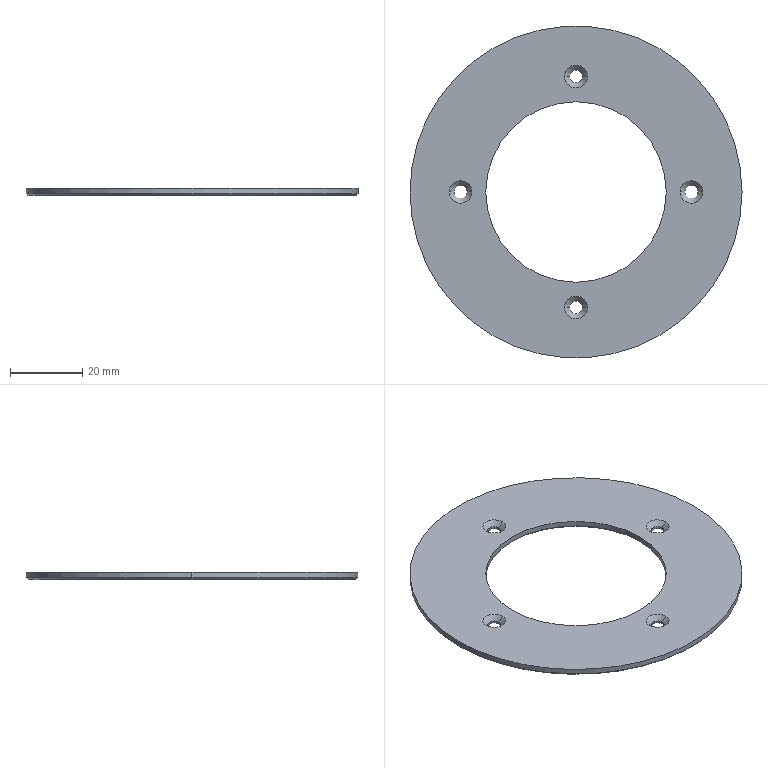Part | NX | features BREP 1 | 1 solid | 26 faces | box 92 x 92 x 2 mm | volume 9180 mm3 | cone 12 | cylinder 12 | plane 2 | commonest cylinder face diameters 3.6 x8 50 x2 92 x2
STEP:
#1=CARTESIAN_POINT('',(-45.5,0.,0.));
#2=VERTEX_POINT('',#1);
#3=CARTESIAN_POINT('',(45.5,0.,0.));
#4=VERTEX_POINT('',#3);
#5=CARTESIAN_POINT('',(0.,0.,0.));
#6=DIRECTION('',(0.,0.,-1.));
#7=DIRECTION('',(1.,0.,0.));
#8=AXIS2_PLACEMENT_3D('',#5,#6,#7);
#9=CIRCLE('',#8,45.5);
#10=EDGE_CURVE('',#2,#4,#9,.T.);
#11=ORIENTED_EDGE('',*,*,#10,.F.);
#12=CARTESIAN_POINT('',(-46.,0.,0.5));
#13=VERTEX_POINT('',#12);
#14=CARTESIAN_POINT('',(-46.,0.,0.5));
#15=DIRECTION('',(-0.7071,0.,0.7071));
#16=VECTOR('',#15,1000.);
#17=LINE('',#14,#16);
#18=EDGE_CURVE('',#13,#2,#17,.F.);
#19=ORIENTED_EDGE('',*,*,#18,.F.);
#20=CARTESIAN_POINT('',(46.,0.,0.5));
#21=VERTEX_POINT('',#20);
#22=CARTESIAN_POINT('',(0.,0.,0.5));
#23=DIRECTION('',(0.,0.,1.));
#24=DIRECTION('',(1.,0.,0.));
#25=AXIS2_PLACEMENT_3D('',#22,#23,#24);
#26=CIRCLE('',#25,46.);
#27=EDGE_CURVE('',#21,#13,#26,.T.);
#28=ORIENTED_EDGE('',*,*,#27,.F.);
#29=CARTESIAN_POINT('',(46.,0.,0.5));
#30=DIRECTION('',(0.7071,0.,0.7071));
#31=VECTOR('',#30,1000.);
#32=LINE('',#29,#31);
#33=EDGE_CURVE('',#21,#4,#32,.F.);
#34=ORIENTED_EDGE('',*,*,#33,.T.);
#35=EDGE_LOOP('',(#11,#19,#28,#34));
#36=FACE_BOUND('',#35,.T.);
#37=CARTESIAN_POINT('',(0.,0.,0.5));
#38=DIRECTION('',(0.,0.,1.));
#39=DIRECTION('',(1.,0.,0.));
#40=AXIS2_PLACEMENT_3D('',#37,#38,#39);
#41=CONICAL_SURFACE('',#40,46.,0.7854);
#42=ADVANCED_FACE('',(#36),#41,.T.);
#43=CARTESIAN_POINT('',(25.,0.,0.5));
#44=VERTEX_POINT('',#43);
#45=CARTESIAN_POINT('',(-25.,0.,0.5));
#46=VERTEX_POINT('',#45);
#47=CARTESIAN_POINT('',(0.,0.,0.5));
#48=DIRECTION('',(0.,0.,-1.));
#49=DIRECTION('',(1.,0.,0.));
#50=AXIS2_PLACEMENT_3D('',#47,#48,#49);
#51=CIRCLE('',#50,25.);
#52=EDGE_CURVE('',#44,#46,#51,.T.);
#53=ORIENTED_EDGE('',*,*,#52,.F.);
#54=CARTESIAN_POINT('',(25.5,0.,0.));
#55=VERTEX_POINT('',#54);
#56=CARTESIAN_POINT('',(25.5,0.,0.));
#57=DIRECTION('',(0.7071,0.,-0.7071));
#58=VECTOR('',#57,1000.);
#59=LINE('',#56,#58);
#60=EDGE_CURVE('',#44,#55,#59,.T.);
#61=ORIENTED_EDGE('',*,*,#60,.T.);
#62=CARTESIAN_POINT('',(-25.5,0.,0.));
#63=VERTEX_POINT('',#62);
#64=CARTESIAN_POINT('',(0.,0.,0.));
#65=DIRECTION('',(0.,0.,1.));
#66=DIRECTION('',(1.,0.,0.));
#67=AXIS2_PLACEMENT_3D('',#64,#65,#66);
#68=CIRCLE('',#67,25.5);
#69=EDGE_CURVE('',#63,#55,#68,.T.);
#70=ORIENTED_EDGE('',*,*,#69,.F.);
#71=CARTESIAN_POINT('',(-25.5,0.,0.));
#72=DIRECTION('',(-0.7071,0.,-0.7071));
#73=VECTOR('',#72,1000.);
#74=LINE('',#71,#73);
#75=EDGE_CURVE('',#46,#63,#74,.T.);
#76=ORIENTED_EDGE('',*,*,#75,.F.);
#77=EDGE_LOOP('',(#53,#61,#70,#76));
#78=FACE_BOUND('',#77,.T.);
#79=CARTESIAN_POINT('',(0.,0.,0.));
#80=DIRECTION('',(0.,0.,-1.));
#81=DIRECTION('',(-1.,0.,0.));
#82=AXIS2_PLACEMENT_3D('',#79,#80,#81);
#83=CONICAL_SURFACE('',#82,25.5,0.7854);
#84=ADVANCED_FACE('',(#78),#83,.F.);
#85=CARTESIAN_POINT('',(-33.8,0.,0.65));
#86=VERTEX_POINT('',#85);
#87=CARTESIAN_POINT('',(-30.2,0.,0.65));
#88=VERTEX_POINT('',#87);
#89=CARTESIAN_POINT('',(-32.,0.,0.65));
#90=DIRECTION('',(0.,0.,1.));
#91=DIRECTION('',(1.,0.,0.));
#92=AXIS2_PLACEMENT_3D('',#89,#90,#91);
#93=CIRCLE('',#92,1.8);
#94=EDGE_CURVE('',#86,#88,#93,.T.);
#95=ORIENTED_EDGE('',*,*,#94,.F.);
#96=CARTESIAN_POINT('',(-35.15,0.,2.));
#97=VERTEX_POINT('',#96);
#98=CARTESIAN_POINT('',(-35.15,0.,2.));
#99=DIRECTION('',(-0.7071,0.,0.7071));
#100=VECTOR('',#99,1000.);
#101=LINE('',#98,#100);
#102=EDGE_CURVE('',#97,#86,#101,.F.);
#103=ORIENTED_EDGE('',*,*,#102,.F.);
#104=CARTESIAN_POINT('',(-28.85,0.,2.));
#105=VERTEX_POINT('',#104);
#106=CARTESIAN_POINT('',(-32.,0.,2.));
#107=DIRECTION('',(0.,0.,1.));
#108=DIRECTION('',(1.,0.,0.));
#109=AXIS2_PLACEMENT_3D('',#106,#107,#108);
#110=CIRCLE('',#109,3.15);
#111=EDGE_CURVE('',#97,#105,#110,.T.);
#112=ORIENTED_EDGE('',*,*,#111,.T.);
#113=CARTESIAN_POINT('',(-28.85,0.,2.));
#114=DIRECTION('',(0.7071,0.,0.7071));
#115=VECTOR('',#114,1000.);
#116=LINE('',#113,#115);
#117=EDGE_CURVE('',#105,#88,#116,.F.);
#118=ORIENTED_EDGE('',*,*,#117,.T.);
#119=EDGE_LOOP('',(#95,#103,#112,#118));
#120=FACE_BOUND('',#119,.T.);
#121=CARTESIAN_POINT('',(-32.,0.,2.));
#122=DIRECTION('',(0.,0.,1.));
#123=DIRECTION('',(1.,0.,0.));
#124=AXIS2_PLACEMENT_3D('',#121,#122,#123);
#125=CONICAL_SURFACE('',#124,3.15,0.7854);
#126=ADVANCED_FACE('',(#120),#125,.F.);
#127=CARTESIAN_POINT('',(-33.8,0.,0.));
#128=VERTEX_POINT('',#127);
#129=CARTESIAN_POINT('',(-30.2,0.,0.));
#130=VERTEX_POINT('',#129);
#131=CARTESIAN_POINT('',(-32.,0.,0.));
#132=DIRECTION('',(0.,0.,1.));
#133=DIRECTION('',(1.,0.,0.));
#134=AXIS2_PLACEMENT_3D('',#131,#132,#133);
#135=CIRCLE('',#134,1.8);
#136=EDGE_CURVE('',#128,#130,#135,.T.);
#137=ORIENTED_EDGE('',*,*,#136,.F.);
#138=CARTESIAN_POINT('',(-33.8,0.,2.));
#139=DIRECTION('',(0.,0.,1.));
#140=VECTOR('',#139,1000.);
#141=LINE('',#138,#140);
#142=EDGE_CURVE('',#86,#128,#141,.F.);
#143=ORIENTED_EDGE('',*,*,#142,.F.);
#144=ORIENTED_EDGE('',*,*,#94,.T.);
#145=CARTESIAN_POINT('',(-30.2,0.,2.));
#146=DIRECTION('',(0.,0.,1.));
#147=VECTOR('',#146,1000.);
#148=LINE('',#145,#147);
#149=EDGE_CURVE('',#88,#130,#148,.F.);
#150=ORIENTED_EDGE('',*,*,#149,.T.);
#151=EDGE_LOOP('',(#137,#143,#144,#150));
#152=FACE_BOUND('',#151,.T.);
#153=CARTESIAN_POINT('',(-32.,0.,2.));
#154=DIRECTION('',(0.,0.,1.));
#155=DIRECTION('',(1.,0.,0.));
#156=AXIS2_PLACEMENT_3D('',#153,#154,#155);
#157=CYLINDRICAL_SURFACE('',#156,1.8);
#158=ADVANCED_FACE('',(#152),#157,.F.);
#159=CARTESIAN_POINT('',(-1.8,-32.,0.65));
#160=VERTEX_POINT('',#159);
#161=CARTESIAN_POINT('',(1.8,-32.,0.65));
#162=VERTEX_POINT('',#161);
#163=CARTESIAN_POINT('',(0.,-32.,0.65));
#164=DIRECTION('',(0.,0.,1.));
#165=DIRECTION('',(1.,0.,0.));
#166=AXIS2_PLACEMENT_3D('',#163,#164,#165);
#167=CIRCLE('',#166,1.8);
#168=EDGE_CURVE('',#160,#162,#167,.T.);
#169=ORIENTED_EDGE('',*,*,#168,.F.);
#170=CARTESIAN_POINT('',(-3.15,-32.,2.));
#171=VERTEX_POINT('',#170);
#172=CARTESIAN_POINT('',(-3.15,-32.,2.));
#173=DIRECTION('',(-0.7071,0.,0.7071));
#174=VECTOR('',#173,1000.);
#175=LINE('',#172,#174);
#176=EDGE_CURVE('',#171,#160,#175,.F.);
#177=ORIENTED_EDGE('',*,*,#176,.F.);
#178=CARTESIAN_POINT('',(3.15,-32.,2.));
#179=VERTEX_POINT('',#178);
#180=CARTESIAN_POINT('',(0.,-32.,2.));
#181=DIRECTION('',(0.,0.,1.));
#182=DIRECTION('',(1.,0.,0.));
#183=AXIS2_PLACEMENT_3D('',#180,#181,#182);
#184=CIRCLE('',#183,3.15);
#185=EDGE_CURVE('',#171,#179,#184,.T.);
#186=ORIENTED_EDGE('',*,*,#185,.T.);
#187=CARTESIAN_POINT('',(3.15,-32.,2.));
#188=DIRECTION('',(0.7071,0.,0.7071));
#189=VECTOR('',#188,1000.);
#190=LINE('',#187,#189);
#191=EDGE_CURVE('',#179,#162,#190,.F.);
#192=ORIENTED_EDGE('',*,*,#191,.T.);
#193=EDGE_LOOP('',(#169,#177,#186,#192));
#194=FACE_BOUND('',#193,.T.);
#195=CARTESIAN_POINT('',(0.,-32.,2.));
#196=DIRECTION('',(0.,0.,1.));
#197=DIRECTION('',(1.,0.,0.));
#198=AXIS2_PLACEMENT_3D('',#195,#196,#197);
#199=CONICAL_SURFACE('',#198,3.15,0.7854);
#200=ADVANCED_FACE('',(#194),#199,.F.);
#201=CARTESIAN_POINT('',(-1.8,-32.,0.));
#202=VERTEX_POINT('',#201);
#203=CARTESIAN_POINT('',(1.8,-32.,0.));
#204=VERTEX_POINT('',#203);
#205=CARTESIAN_POINT('',(0.,-32.,0.));
#206=DIRECTION('',(0.,0.,1.));
#207=DIRECTION('',(1.,0.,0.));
#208=AXIS2_PLACEMENT_3D('',#205,#206,#207);
#209=CIRCLE('',#208,1.8);
#210=EDGE_CURVE('',#202,#204,#209,.T.);
#211=ORIENTED_EDGE('',*,*,#210,.F.);
#212=CARTESIAN_POINT('',(-1.8,-32.,2.));
#213=DIRECTION('',(0.,0.,1.));
#214=VECTOR('',#213,1000.);
#215=LINE('',#212,#214);
#216=EDGE_CURVE('',#160,#202,#215,.F.);
#217=ORIENTED_EDGE('',*,*,#216,.F.);
#218=ORIENTED_EDGE('',*,*,#168,.T.);
#219=CARTESIAN_POINT('',(1.8,-32.,2.));
#220=DIRECTION('',(0.,0.,1.));
#221=VECTOR('',#220,1000.);
#222=LINE('',#219,#221);
#223=EDGE_CURVE('',#162,#204,#222,.F.);
#224=ORIENTED_EDGE('',*,*,#223,.T.);
#225=EDGE_LOOP('',(#211,#217,#218,#224));
#226=FACE_BOUND('',#225,.T.);
#227=CARTESIAN_POINT('',(0.,-32.,2.));
#228=DIRECTION('',(0.,0.,1.));
#229=DIRECTION('',(1.,0.,0.));
#230=AXIS2_PLACEMENT_3D('',#227,#228,#229);
#231=CYLINDRICAL_SURFACE('',#230,1.8);
#232=ADVANCED_FACE('',(#226),#231,.F.);
#233=CARTESIAN_POINT('',(30.2,0.,0.65));
#234=VERTEX_POINT('',#233);
#235=CARTESIAN_POINT('',(33.8,0.,0.65));
#236=VERTEX_POINT('',#235);
#237=CARTESIAN_POINT('',(32.,0.,0.65));
#238=DIRECTION('',(0.,0.,1.));
#239=DIRECTION('',(1.,0.,0.));
#240=AXIS2_PLACEMENT_3D('',#237,#238,#239);
#241=CIRCLE('',#240,1.8);
#242=EDGE_CURVE('',#234,#236,#241,.T.);
#243=ORIENTED_EDGE('',*,*,#242,.F.);
#244=CARTESIAN_POINT('',(28.85,0.,2.));
#245=VERTEX_POINT('',#244);
#246=CARTESIAN_POINT('',(28.85,0.,2.));
#247=DIRECTION('',(-0.7071,0.,0.7071));
#248=VECTOR('',#247,1000.);
#249=LINE('',#246,#248);
#250=EDGE_CURVE('',#245,#234,#249,.F.);
#251=ORIENTED_EDGE('',*,*,#250,.F.);
#252=CARTESIAN_POINT('',(35.15,0.,2.));
#253=VERTEX_POINT('',#252);
#254=CARTESIAN_POINT('',(32.,0.,2.));
#255=DIRECTION('',(0.,0.,1.));
#256=DIRECTION('',(1.,0.,0.));
#257=AXIS2_PLACEMENT_3D('',#254,#255,#256);
#258=CIRCLE('',#257,3.15);
#259=EDGE_CURVE('',#245,#253,#258,.T.);
#260=ORIENTED_EDGE('',*,*,#259,.T.);
#261=CARTESIAN_POINT('',(35.15,0.,2.));
#262=DIRECTION('',(0.7071,0.,0.7071));
#263=VECTOR('',#262,1000.);
#264=LINE('',#261,#263);
#265=EDGE_CURVE('',#253,#236,#264,.F.);
#266=ORIENTED_EDGE('',*,*,#265,.T.);
#267=EDGE_LOOP('',(#243,#251,#260,#266));
#268=FACE_BOUND('',#267,.T.);
#269=CARTESIAN_POINT('',(32.,0.,2.));
#270=DIRECTION('',(0.,0.,1.));
#271=DIRECTION('',(1.,0.,0.));
#272=AXIS2_PLACEMENT_3D('',#269,#270,#271);
#273=CONICAL_SURFACE('',#272,3.15,0.7854);
#274=ADVANCED_FACE('',(#268),#273,.F.);
#275=CARTESIAN_POINT('',(30.2,0.,0.));
#276=VERTEX_POINT('',#275);
#277=CARTESIAN_POINT('',(33.8,0.,0.));
#278=VERTEX_POINT('',#277);
#279=CARTESIAN_POINT('',(32.,0.,0.));
#280=DIRECTION('',(0.,0.,1.));
#281=DIRECTION('',(1.,0.,0.));
#282=AXIS2_PLACEMENT_3D('',#279,#280,#281);
#283=CIRCLE('',#282,1.8);
#284=EDGE_CURVE('',#276,#278,#283,.T.);
#285=ORIENTED_EDGE('',*,*,#284,.F.);
#286=CARTESIAN_POINT('',(30.2,0.,2.));
#287=DIRECTION('',(0.,0.,1.));
#288=VECTOR('',#287,1000.);
#289=LINE('',#286,#288);
#290=EDGE_CURVE('',#234,#276,#289,.F.);
#291=ORIENTED_EDGE('',*,*,#290,.F.);
#292=ORIENTED_EDGE('',*,*,#242,.T.);
#293=CARTESIAN_POINT('',(33.8,0.,2.));
#294=DIRECTION('',(0.,0.,1.));
#295=VECTOR('',#294,1000.);
#296=LINE('',#293,#295);
#297=EDGE_CURVE('',#236,#278,#296,.F.);
#298=ORIENTED_EDGE('',*,*,#297,.T.);
#299=EDGE_LOOP('',(#285,#291,#292,#298));
#300=FACE_BOUND('',#299,.T.);
#301=CARTESIAN_POINT('',(32.,0.,2.));
#302=DIRECTION('',(0.,0.,1.));
#303=DIRECTION('',(1.,0.,0.));
#304=AXIS2_PLACEMENT_3D('',#301,#302,#303);
#305=CYLINDRICAL_SURFACE('',#304,1.8);
#306=ADVANCED_FACE('',(#300),#305,.F.);
#307=CARTESIAN_POINT('',(-1.8,32.,0.65));
#308=VERTEX_POINT('',#307);
#309=CARTESIAN_POINT('',(1.8,32.,0.65));
#310=VERTEX_POINT('',#309);
#311=CARTESIAN_POINT('',(0.,32.,0.65));
#312=DIRECTION('',(0.,0.,1.));
#313=DIRECTION('',(1.,0.,0.));
#314=AXIS2_PLACEMENT_3D('',#311,#312,#313);
#315=CIRCLE('',#314,1.8);
#316=EDGE_CURVE('',#308,#310,#315,.T.);
#317=ORIENTED_EDGE('',*,*,#316,.F.);
#318=CARTESIAN_POINT('',(-3.15,32.,2.));
#319=VERTEX_POINT('',#318);
#320=CARTESIAN_POINT('',(-3.15,32.,2.));
#321=DIRECTION('',(-0.7071,0.,0.7071));
#322=VECTOR('',#321,1000.);
#323=LINE('',#320,#322);
#324=EDGE_CURVE('',#319,#308,#323,.F.);
#325=ORIENTED_EDGE('',*,*,#324,.F.);
#326=CARTESIAN_POINT('',(3.15,32.,2.));
#327=VERTEX_POINT('',#326);
#328=CARTESIAN_POINT('',(0.,32.,2.));
#329=DIRECTION('',(0.,0.,1.));
#330=DIRECTION('',(1.,0.,0.));
#331=AXIS2_PLACEMENT_3D('',#328,#329,#330);
#332=CIRCLE('',#331,3.15);
#333=EDGE_CURVE('',#319,#327,#332,.T.);
#334=ORIENTED_EDGE('',*,*,#333,.T.);
#335=CARTESIAN_POINT('',(3.15,32.,2.));
#336=DIRECTION('',(0.7071,0.,0.7071));
#337=VECTOR('',#336,1000.);
#338=LINE('',#335,#337);
#339=EDGE_CURVE('',#327,#310,#338,.F.);
#340=ORIENTED_EDGE('',*,*,#339,.T.);
#341=EDGE_LOOP('',(#317,#325,#334,#340));
#342=FACE_BOUND('',#341,.T.);
#343=CARTESIAN_POINT('',(0.,32.,2.));
#344=DIRECTION('',(0.,0.,1.));
#345=DIRECTION('',(1.,0.,0.));
#346=AXIS2_PLACEMENT_3D('',#343,#344,#345);
#347=CONICAL_SURFACE('',#346,3.15,0.7854);
#348=ADVANCED_FACE('',(#342),#347,.F.);
#349=CARTESIAN_POINT('',(-1.8,32.,0.));
#350=VERTEX_POINT('',#349);
#351=CARTESIAN_POINT('',(1.8,32.,0.));
#352=VERTEX_POINT('',#351);
#353=CARTESIAN_POINT('',(0.,32.,0.));
#354=DIRECTION('',(0.,0.,1.));
#355=DIRECTION('',(1.,0.,0.));
#356=AXIS2_PLACEMENT_3D('',#353,#354,#355);
#357=CIRCLE('',#356,1.8);
#358=EDGE_CURVE('',#350,#352,#357,.T.);
#359=ORIENTED_EDGE('',*,*,#358,.F.);
#360=CARTESIAN_POINT('',(-1.8,32.,2.));
#361=DIRECTION('',(0.,0.,1.));
#362=VECTOR('',#361,1000.);
#363=LINE('',#360,#362);
#364=EDGE_CURVE('',#308,#350,#363,.F.);
#365=ORIENTED_EDGE('',*,*,#364,.F.);
#366=ORIENTED_EDGE('',*,*,#316,.T.);
#367=CARTESIAN_POINT('',(1.8,32.,2.));
#368=DIRECTION('',(0.,0.,1.));
#369=VECTOR('',#368,1000.);
#370=LINE('',#367,#369);
#371=EDGE_CURVE('',#310,#352,#370,.F.);
#372=ORIENTED_EDGE('',*,*,#371,.T.);
#373=EDGE_LOOP('',(#359,#365,#366,#372));
#374=FACE_BOUND('',#373,.T.);
#375=CARTESIAN_POINT('',(0.,32.,2.));
#376=DIRECTION('',(0.,0.,1.));
#377=DIRECTION('',(1.,0.,0.));
#378=AXIS2_PLACEMENT_3D('',#375,#376,#377);
#379=CYLINDRICAL_SURFACE('',#378,1.8);
#380=ADVANCED_FACE('',(#374),#379,.F.);
#381=CARTESIAN_POINT('',(-25.,0.,2.));
#382=VERTEX_POINT('',#381);
#383=CARTESIAN_POINT('',(25.,0.,2.));
#384=VERTEX_POINT('',#383);
#385=CARTESIAN_POINT('',(0.,0.,2.));
#386=DIRECTION('',(0.,0.,1.));
#387=DIRECTION('',(1.,0.,0.));
#388=AXIS2_PLACEMENT_3D('',#385,#386,#387);
#389=CIRCLE('',#388,25.);
#390=EDGE_CURVE('',#382,#384,#389,.T.);
#391=ORIENTED_EDGE('',*,*,#390,.T.);
#392=CARTESIAN_POINT('',(25.,0.,2.));
#393=DIRECTION('',(0.,0.,-1.));
#394=VECTOR('',#393,1000.);
#395=LINE('',#392,#394);
#396=EDGE_CURVE('',#384,#44,#395,.T.);
#397=ORIENTED_EDGE('',*,*,#396,.T.);
#398=ORIENTED_EDGE('',*,*,#52,.T.);
#399=CARTESIAN_POINT('',(-25.,0.,2.));
#400=DIRECTION('',(0.,0.,-1.));
#401=VECTOR('',#400,1000.);
#402=LINE('',#399,#401);
#403=EDGE_CURVE('',#382,#46,#402,.T.);
#404=ORIENTED_EDGE('',*,*,#403,.F.);
#405=EDGE_LOOP('',(#391,#397,#398,#404));
#406=FACE_BOUND('',#405,.T.);
#407=CARTESIAN_POINT('',(0.,0.,2.));
#408=DIRECTION('',(0.,0.,-1.));
#409=DIRECTION('',(-1.,0.,0.));
#410=AXIS2_PLACEMENT_3D('',#407,#408,#409);
#411=CYLINDRICAL_SURFACE('',#410,25.);
#412=ADVANCED_FACE('',(#406),#411,.F.);
#413=CARTESIAN_POINT('',(46.,0.,2.));
#414=VERTEX_POINT('',#413);
#415=CARTESIAN_POINT('',(-46.,0.,2.));
#416=VERTEX_POINT('',#415);
#417=CARTESIAN_POINT('',(0.,0.,2.));
#418=DIRECTION('',(0.,0.,1.));
#419=DIRECTION('',(1.,0.,0.));
#420=AXIS2_PLACEMENT_3D('',#417,#418,#419);
#421=CIRCLE('',#420,46.);
#422=EDGE_CURVE('',#414,#416,#421,.T.);
#423=ORIENTED_EDGE('',*,*,#422,.F.);
#424=CARTESIAN_POINT('',(46.,0.,2.));
#425=DIRECTION('',(0.,0.,-1.));
#426=VECTOR('',#425,1000.);
#427=LINE('',#424,#426);
#428=EDGE_CURVE('',#414,#21,#427,.T.);
#429=ORIENTED_EDGE('',*,*,#428,.T.);
#430=ORIENTED_EDGE('',*,*,#27,.T.);
#431=CARTESIAN_POINT('',(-46.,0.,2.));
#432=DIRECTION('',(0.,0.,-1.));
#433=VECTOR('',#432,1000.);
#434=LINE('',#431,#433);
#435=EDGE_CURVE('',#416,#13,#434,.T.);
#436=ORIENTED_EDGE('',*,*,#435,.F.);
#437=EDGE_LOOP('',(#423,#429,#430,#436));
#438=FACE_BOUND('',#437,.T.);
#439=CARTESIAN_POINT('',(0.,0.,2.));
#440=DIRECTION('',(0.,0.,-1.));
#441=DIRECTION('',(-1.,0.,0.));
#442=AXIS2_PLACEMENT_3D('',#439,#440,#441);
#443=CYLINDRICAL_SURFACE('',#442,46.);
#444=ADVANCED_FACE('',(#438),#443,.T.);
#445=CARTESIAN_POINT('',(0.,0.,2.));
#446=DIRECTION('',(0.,0.,1.));
#447=DIRECTION('',(1.,0.,0.));
#448=AXIS2_PLACEMENT_3D('',#445,#446,#447);
#449=CIRCLE('',#448,46.);
#450=EDGE_CURVE('',#416,#414,#449,.T.);
#451=ORIENTED_EDGE('',*,*,#450,.T.);
#452=ORIENTED_EDGE('',*,*,#422,.T.);
#453=EDGE_LOOP('',(#451,#452));
#454=FACE_BOUND('',#453,.T.);
#455=CARTESIAN_POINT('',(-32.,0.,2.));
#456=DIRECTION('',(0.,0.,1.));
#457=DIRECTION('',(1.,0.,0.));
#458=AXIS2_PLACEMENT_3D('',#455,#456,#457);
#459=CIRCLE('',#458,3.15);
#460=EDGE_CURVE('',#105,#97,#459,.T.);
#461=ORIENTED_EDGE('',*,*,#460,.F.);
#462=ORIENTED_EDGE('',*,*,#111,.F.);
#463=EDGE_LOOP('',(#461,#462));
#464=FACE_BOUND('',#463,.T.);
#465=CARTESIAN_POINT('',(0.,-32.,2.));
#466=DIRECTION('',(0.,0.,1.));
#467=DIRECTION('',(1.,0.,0.));
#468=AXIS2_PLACEMENT_3D('',#465,#466,#467);
#469=CIRCLE('',#468,3.15);
#470=EDGE_CURVE('',#179,#171,#469,.T.);
#471=ORIENTED_EDGE('',*,*,#470,.F.);
#472=ORIENTED_EDGE('',*,*,#185,.F.);
#473=EDGE_LOOP('',(#471,#472));
#474=FACE_BOUND('',#473,.T.);
#475=CARTESIAN_POINT('',(32.,0.,2.));
#476=DIRECTION('',(0.,0.,1.));
#477=DIRECTION('',(1.,0.,0.));
#478=AXIS2_PLACEMENT_3D('',#475,#476,#477);
#479=CIRCLE('',#478,3.15);
#480=EDGE_CURVE('',#253,#245,#479,.T.);
#481=ORIENTED_EDGE('',*,*,#480,.F.);
#482=ORIENTED_EDGE('',*,*,#259,.F.);
#483=EDGE_LOOP('',(#481,#482));
#484=FACE_BOUND('',#483,.T.);
#485=CARTESIAN_POINT('',(0.,32.,2.));
#486=DIRECTION('',(0.,0.,1.));
#487=DIRECTION('',(1.,0.,0.));
#488=AXIS2_PLACEMENT_3D('',#485,#486,#487);
#489=CIRCLE('',#488,3.15);
#490=EDGE_CURVE('',#327,#319,#489,.T.);
#491=ORIENTED_EDGE('',*,*,#490,.F.);
#492=ORIENTED_EDGE('',*,*,#333,.F.);
#493=EDGE_LOOP('',(#491,#492));
#494=FACE_BOUND('',#493,.T.);
#495=ORIENTED_EDGE('',*,*,#390,.F.);
#496=CARTESIAN_POINT('',(0.,0.,2.));
#497=DIRECTION('',(0.,0.,1.));
#498=DIRECTION('',(1.,0.,0.));
#499=AXIS2_PLACEMENT_3D('',#496,#497,#498);
#500=CIRCLE('',#499,25.);
#501=EDGE_CURVE('',#384,#382,#500,.T.);
#502=ORIENTED_EDGE('',*,*,#501,.F.);
#503=EDGE_LOOP('',(#495,#502));
#504=FACE_BOUND('',#503,.T.);
#505=CARTESIAN_POINT('',(0.,0.,2.));
#506=DIRECTION('',(0.,0.,1.));
#507=DIRECTION('',(1.,0.,0.));
#508=AXIS2_PLACEMENT_3D('',#505,#506,#507);
#509=PLANE('',#508);
#510=ADVANCED_FACE('',(#454,#464,#474,#484,#494,#504),#509,.T.);
#511=CARTESIAN_POINT('',(0.,0.,0.));
#512=DIRECTION('',(0.,0.,-1.));
#513=DIRECTION('',(1.,0.,0.));
#514=AXIS2_PLACEMENT_3D('',#511,#512,#513);
#515=CIRCLE('',#514,45.5);
#516=EDGE_CURVE('',#4,#2,#515,.T.);
#517=ORIENTED_EDGE('',*,*,#516,.T.);
#518=ORIENTED_EDGE('',*,*,#10,.T.);
#519=EDGE_LOOP('',(#517,#518));
#520=FACE_BOUND('',#519,.T.);
#521=ORIENTED_EDGE('',*,*,#69,.T.);
#522=CARTESIAN_POINT('',(0.,0.,0.));
#523=DIRECTION('',(0.,0.,1.));
#524=DIRECTION('',(1.,0.,0.));
#525=AXIS2_PLACEMENT_3D('',#522,#523,#524);
#526=CIRCLE('',#525,25.5);
#527=EDGE_CURVE('',#55,#63,#526,.T.);
#528=ORIENTED_EDGE('',*,*,#527,.T.);
#529=EDGE_LOOP('',(#521,#528));
#530=FACE_BOUND('',#529,.T.);
#531=CARTESIAN_POINT('',(-32.,0.,0.));
#532=DIRECTION('',(0.,0.,1.));
#533=DIRECTION('',(1.,0.,0.));
#534=AXIS2_PLACEMENT_3D('',#531,#532,#533);
#535=CIRCLE('',#534,1.8);
#536=EDGE_CURVE('',#130,#128,#535,.T.);
#537=ORIENTED_EDGE('',*,*,#536,.T.);
#538=ORIENTED_EDGE('',*,*,#136,.T.);
#539=EDGE_LOOP('',(#537,#538));
#540=FACE_BOUND('',#539,.T.);
#541=CARTESIAN_POINT('',(0.,-32.,0.));
#542=DIRECTION('',(0.,0.,1.));
#543=DIRECTION('',(1.,0.,0.));
#544=AXIS2_PLACEMENT_3D('',#541,#542,#543);
#545=CIRCLE('',#544,1.8);
#546=EDGE_CURVE('',#204,#202,#545,.T.);
#547=ORIENTED_EDGE('',*,*,#546,.T.);
#548=ORIENTED_EDGE('',*,*,#210,.T.);
#549=EDGE_LOOP('',(#547,#548));
#550=FACE_BOUND('',#549,.T.);
#551=CARTESIAN_POINT('',(32.,0.,0.));
#552=DIRECTION('',(0.,0.,1.));
#553=DIRECTION('',(1.,0.,0.));
#554=AXIS2_PLACEMENT_3D('',#551,#552,#553);
#555=CIRCLE('',#554,1.8);
#556=EDGE_CURVE('',#278,#276,#555,.T.);
#557=ORIENTED_EDGE('',*,*,#556,.T.);
#558=ORIENTED_EDGE('',*,*,#284,.T.);
#559=EDGE_LOOP('',(#557,#558));
#560=FACE_BOUND('',#559,.T.);
#561=CARTESIAN_POINT('',(0.,32.,0.));
#562=DIRECTION('',(0.,0.,1.));
#563=DIRECTION('',(1.,0.,0.));
#564=AXIS2_PLACEMENT_3D('',#561,#562,#563);
#565=CIRCLE('',#564,1.8);
#566=EDGE_CURVE('',#352,#350,#565,.T.);
#567=ORIENTED_EDGE('',*,*,#566,.T.);
#568=ORIENTED_EDGE('',*,*,#358,.T.);
#569=EDGE_LOOP('',(#567,#568));
#570=FACE_BOUND('',#569,.T.);
#571=CARTESIAN_POINT('',(0.,0.,0.));
#572=DIRECTION('',(0.,0.,1.));
#573=DIRECTION('',(1.,0.,0.));
#574=AXIS2_PLACEMENT_3D('',#571,#572,#573);
#575=PLANE('',#574);
#576=ADVANCED_FACE('',(#520,#530,#540,#550,#560,#570),#575,.F.);
#577=ORIENTED_EDGE('',*,*,#428,.F.);
#578=ORIENTED_EDGE('',*,*,#450,.F.);
#579=ORIENTED_EDGE('',*,*,#435,.T.);
#580=CARTESIAN_POINT('',(0.,0.,0.5));
#581=DIRECTION('',(0.,0.,1.));
#582=DIRECTION('',(1.,0.,0.));
#583=AXIS2_PLACEMENT_3D('',#580,#581,#582);
#584=CIRCLE('',#583,46.);
#585=EDGE_CURVE('',#13,#21,#584,.T.);
#586=ORIENTED_EDGE('',*,*,#585,.T.);
#587=EDGE_LOOP('',(#577,#578,#579,#586));
#588=FACE_BOUND('',#587,.T.);
#589=CARTESIAN_POINT('',(0.,0.,2.));
#590=DIRECTION('',(0.,0.,-1.));
#591=DIRECTION('',(-1.,0.,0.));
#592=AXIS2_PLACEMENT_3D('',#589,#590,#591);
#593=CYLINDRICAL_SURFACE('',#592,46.);
#594=ADVANCED_FACE('',(#588),#593,.T.);
#595=ORIENTED_EDGE('',*,*,#396,.F.);
#596=ORIENTED_EDGE('',*,*,#501,.T.);
#597=ORIENTED_EDGE('',*,*,#403,.T.);
#598=CARTESIAN_POINT('',(0.,0.,0.5));
#599=DIRECTION('',(0.,0.,-1.));
#600=DIRECTION('',(1.,0.,0.));
#601=AXIS2_PLACEMENT_3D('',#598,#599,#600);
#602=CIRCLE('',#601,25.);
#603=EDGE_CURVE('',#46,#44,#602,.T.);
#604=ORIENTED_EDGE('',*,*,#603,.T.);
#605=EDGE_LOOP('',(#595,#596,#597,#604));
#606=FACE_BOUND('',#605,.T.);
#607=CARTESIAN_POINT('',(0.,0.,2.));
#608=DIRECTION('',(0.,0.,-1.));
#609=DIRECTION('',(-1.,0.,0.));
#610=AXIS2_PLACEMENT_3D('',#607,#608,#609);
#611=CYLINDRICAL_SURFACE('',#610,25.);
#612=ADVANCED_FACE('',(#606),#611,.F.);
#613=ORIENTED_EDGE('',*,*,#364,.T.);
#614=ORIENTED_EDGE('',*,*,#566,.F.);
#615=ORIENTED_EDGE('',*,*,#371,.F.);
#616=CARTESIAN_POINT('',(0.,32.,0.65));
#617=DIRECTION('',(0.,0.,1.));
#618=DIRECTION('',(1.,0.,0.));
#619=AXIS2_PLACEMENT_3D('',#616,#617,#618);
#620=CIRCLE('',#619,1.8);
#621=EDGE_CURVE('',#310,#308,#620,.T.);
#622=ORIENTED_EDGE('',*,*,#621,.T.);
#623=EDGE_LOOP('',(#613,#614,#615,#622));
#624=FACE_BOUND('',#623,.T.);
#625=CARTESIAN_POINT('',(0.,32.,2.));
#626=DIRECTION('',(0.,0.,1.));
#627=DIRECTION('',(1.,0.,0.));
#628=AXIS2_PLACEMENT_3D('',#625,#626,#627);
#629=CYLINDRICAL_SURFACE('',#628,1.8);
#630=ADVANCED_FACE('',(#624),#629,.F.);
#631=ORIENTED_EDGE('',*,*,#324,.T.);
#632=ORIENTED_EDGE('',*,*,#621,.F.);
#633=ORIENTED_EDGE('',*,*,#339,.F.);
#634=ORIENTED_EDGE('',*,*,#490,.T.);
#635=EDGE_LOOP('',(#631,#632,#633,#634));
#636=FACE_BOUND('',#635,.T.);
#637=CARTESIAN_POINT('',(0.,32.,2.));
#638=DIRECTION('',(0.,0.,1.));
#639=DIRECTION('',(1.,0.,0.));
#640=AXIS2_PLACEMENT_3D('',#637,#638,#639);
#641=CONICAL_SURFACE('',#640,3.15,0.7854);
#642=ADVANCED_FACE('',(#636),#641,.F.);
#643=ORIENTED_EDGE('',*,*,#290,.T.);
#644=ORIENTED_EDGE('',*,*,#556,.F.);
#645=ORIENTED_EDGE('',*,*,#297,.F.);
#646=CARTESIAN_POINT('',(32.,0.,0.65));
#647=DIRECTION('',(0.,0.,1.));
#648=DIRECTION('',(1.,0.,0.));
#649=AXIS2_PLACEMENT_3D('',#646,#647,#648);
#650=CIRCLE('',#649,1.8);
#651=EDGE_CURVE('',#236,#234,#650,.T.);
#652=ORIENTED_EDGE('',*,*,#651,.T.);
#653=EDGE_LOOP('',(#643,#644,#645,#652));
#654=FACE_BOUND('',#653,.T.);
#655=CARTESIAN_POINT('',(32.,0.,2.));
#656=DIRECTION('',(0.,0.,1.));
#657=DIRECTION('',(1.,0.,0.));
#658=AXIS2_PLACEMENT_3D('',#655,#656,#657);
#659=CYLINDRICAL_SURFACE('',#658,1.8);
#660=ADVANCED_FACE('',(#654),#659,.F.);
#661=ORIENTED_EDGE('',*,*,#250,.T.);
#662=ORIENTED_EDGE('',*,*,#651,.F.);
#663=ORIENTED_EDGE('',*,*,#265,.F.);
#664=ORIENTED_EDGE('',*,*,#480,.T.);
#665=EDGE_LOOP('',(#661,#662,#663,#664));
#666=FACE_BOUND('',#665,.T.);
#667=CARTESIAN_POINT('',(32.,0.,2.));
#668=DIRECTION('',(0.,0.,1.));
#669=DIRECTION('',(1.,0.,0.));
#670=AXIS2_PLACEMENT_3D('',#667,#668,#669);
#671=CONICAL_SURFACE('',#670,3.15,0.7854);
#672=ADVANCED_FACE('',(#666),#671,.F.);
#673=ORIENTED_EDGE('',*,*,#216,.T.);
#674=ORIENTED_EDGE('',*,*,#546,.F.);
#675=ORIENTED_EDGE('',*,*,#223,.F.);
#676=CARTESIAN_POINT('',(0.,-32.,0.65));
#677=DIRECTION('',(0.,0.,1.));
#678=DIRECTION('',(1.,0.,0.));
#679=AXIS2_PLACEMENT_3D('',#676,#677,#678);
#680=CIRCLE('',#679,1.8);
#681=EDGE_CURVE('',#162,#160,#680,.T.);
#682=ORIENTED_EDGE('',*,*,#681,.T.);
#683=EDGE_LOOP('',(#673,#674,#675,#682));
#684=FACE_BOUND('',#683,.T.);
#685=CARTESIAN_POINT('',(0.,-32.,2.));
#686=DIRECTION('',(0.,0.,1.));
#687=DIRECTION('',(1.,0.,0.));
#688=AXIS2_PLACEMENT_3D('',#685,#686,#687);
#689=CYLINDRICAL_SURFACE('',#688,1.8);
#690=ADVANCED_FACE('',(#684),#689,.F.);
#691=ORIENTED_EDGE('',*,*,#176,.T.);
#692=ORIENTED_EDGE('',*,*,#681,.F.);
#693=ORIENTED_EDGE('',*,*,#191,.F.);
#694=ORIENTED_EDGE('',*,*,#470,.T.);
#695=EDGE_LOOP('',(#691,#692,#693,#694));
#696=FACE_BOUND('',#695,.T.);
#697=CARTESIAN_POINT('',(0.,-32.,2.));
#698=DIRECTION('',(0.,0.,1.));
#699=DIRECTION('',(1.,0.,0.));
#700=AXIS2_PLACEMENT_3D('',#697,#698,#699);
#701=CONICAL_SURFACE('',#700,3.15,0.7854);
#702=ADVANCED_FACE('',(#696),#701,.F.);
#703=ORIENTED_EDGE('',*,*,#142,.T.);
#704=ORIENTED_EDGE('',*,*,#536,.F.);
#705=ORIENTED_EDGE('',*,*,#149,.F.);
#706=CARTESIAN_POINT('',(-32.,0.,0.65));
#707=DIRECTION('',(0.,0.,1.));
#708=DIRECTION('',(1.,0.,0.));
#709=AXIS2_PLACEMENT_3D('',#706,#707,#708);
#710=CIRCLE('',#709,1.8);
#711=EDGE_CURVE('',#88,#86,#710,.T.);
#712=ORIENTED_EDGE('',*,*,#711,.T.);
#713=EDGE_LOOP('',(#703,#704,#705,#712));
#714=FACE_BOUND('',#713,.T.);
#715=CARTESIAN_POINT('',(-32.,0.,2.));
#716=DIRECTION('',(0.,0.,1.));
#717=DIRECTION('',(1.,0.,0.));
#718=AXIS2_PLACEMENT_3D('',#715,#716,#717);
#719=CYLINDRICAL_SURFACE('',#718,1.8);
#720=ADVANCED_FACE('',(#714),#719,.F.);
#721=ORIENTED_EDGE('',*,*,#102,.T.);
#722=ORIENTED_EDGE('',*,*,#711,.F.);
#723=ORIENTED_EDGE('',*,*,#117,.F.);
#724=ORIENTED_EDGE('',*,*,#460,.T.);
#725=EDGE_LOOP('',(#721,#722,#723,#724));
#726=FACE_BOUND('',#725,.T.);
#727=CARTESIAN_POINT('',(-32.,0.,2.));
#728=DIRECTION('',(0.,0.,1.));
#729=DIRECTION('',(1.,0.,0.));
#730=AXIS2_PLACEMENT_3D('',#727,#728,#729);
#731=CONICAL_SURFACE('',#730,3.15,0.7854);
#732=ADVANCED_FACE('',(#726),#731,.F.);
#733=ORIENTED_EDGE('',*,*,#60,.F.);
#734=ORIENTED_EDGE('',*,*,#603,.F.);
#735=ORIENTED_EDGE('',*,*,#75,.T.);
#736=ORIENTED_EDGE('',*,*,#527,.F.);
#737=EDGE_LOOP('',(#733,#734,#735,#736));
#738=FACE_BOUND('',#737,.T.);
#739=CARTESIAN_POINT('',(0.,0.,0.));
#740=DIRECTION('',(0.,0.,-1.));
#741=DIRECTION('',(-1.,0.,0.));
#742=AXIS2_PLACEMENT_3D('',#739,#740,#741);
#743=CONICAL_SURFACE('',#742,25.5,0.7854);
#744=ADVANCED_FACE('',(#738),#743,.F.);
#745=ORIENTED_EDGE('',*,*,#18,.T.);
#746=ORIENTED_EDGE('',*,*,#516,.F.);
#747=ORIENTED_EDGE('',*,*,#33,.F.);
#748=ORIENTED_EDGE('',*,*,#585,.F.);
#749=EDGE_LOOP('',(#745,#746,#747,#748));
#750=FACE_BOUND('',#749,.T.);
#751=CARTESIAN_POINT('',(0.,0.,0.5));
#752=DIRECTION('',(0.,0.,1.));
#753=DIRECTION('',(1.,0.,0.));
#754=AXIS2_PLACEMENT_3D('',#751,#752,#753);
#755=CONICAL_SURFACE('',#754,46.,0.7854);
#756=ADVANCED_FACE('',(#750),#755,.T.);
#757=CLOSED_SHELL('',(#42,#84,#126,#158,#200,#232,#274,#306,#348,#380,#412,#444,#510,#576,#594,#612,#630,#642,#660,#672,#690,#702,#720,#732,#744,#756));
#758=MANIFOLD_SOLID_BREP('',#757);
#759=(LENGTH_UNIT()NAMED_UNIT(*)SI_UNIT(.MILLI.,.METRE.));
#760=UNCERTAINTY_MEASURE_WITH_UNIT(LENGTH_MEASURE(0.00001),#759,'','');
#761=(NAMED_UNIT(*)PLANE_ANGLE_UNIT()SI_UNIT($,.RADIAN.));
#762=(NAMED_UNIT(*)SI_UNIT($,.STERADIAN.)SOLID_ANGLE_UNIT());
#763=(GEOMETRIC_REPRESENTATION_CONTEXT(3)GLOBAL_UNCERTAINTY_ASSIGNED_CONTEXT((#760))GLOBAL_UNIT_ASSIGNED_CONTEXT((#759,#761,#762))REPRESENTATION_CONTEXT('',''));
#764=ADVANCED_BREP_SHAPE_REPRESENTATION('',(#758),#763);